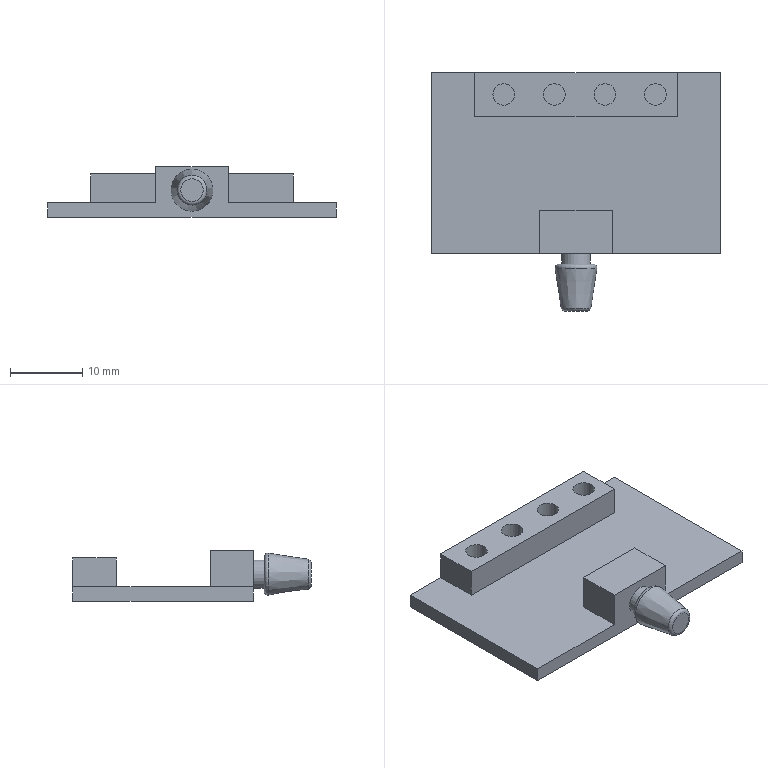Part | NX | features DATUM_CSYS 6, EXTRUDE 5, SKETCH 5, BLEND 2, CHAMFER 1 | 1 solid | 28 faces | box 40 x 33 x 7 mm | volume 3005 mm3 | plane 20 | cylinder 5 | torus 2 | cone 1 | commonest cylinder face diameters 3 x4 4 x1
STEP:
#1=CARTESIAN_POINT('',(-20.,12.5,2.));
#2=VERTEX_POINT('',#1);
#3=CARTESIAN_POINT('',(-20.,-12.5,2.));
#4=VERTEX_POINT('',#3);
#5=CARTESIAN_POINT('',(-20.,12.5,2.));
#6=DIRECTION('',(0.,-1.,0.));
#7=VECTOR('',#6,1000.);
#8=LINE('',#5,#7);
#9=EDGE_CURVE('',#2,#4,#8,.T.);
#10=ORIENTED_EDGE('',*,*,#9,.F.);
#11=CARTESIAN_POINT('',(-20.,12.5,0.));
#12=VERTEX_POINT('',#11);
#13=CARTESIAN_POINT('',(-20.,12.5,0.));
#14=DIRECTION('',(0.,0.,1.));
#15=VECTOR('',#14,1000.);
#16=LINE('',#13,#15);
#17=EDGE_CURVE('',#12,#2,#16,.T.);
#18=ORIENTED_EDGE('',*,*,#17,.F.);
#19=CARTESIAN_POINT('',(-20.,-12.5,0.));
#20=VERTEX_POINT('',#19);
#21=CARTESIAN_POINT('',(-20.,12.5,0.));
#22=DIRECTION('',(0.,-1.,0.));
#23=VECTOR('',#22,1000.);
#24=LINE('',#21,#23);
#25=EDGE_CURVE('',#12,#20,#24,.T.);
#26=ORIENTED_EDGE('',*,*,#25,.T.);
#27=CARTESIAN_POINT('',(-20.,-12.5,0.));
#28=DIRECTION('',(0.,0.,1.));
#29=VECTOR('',#28,1000.);
#30=LINE('',#27,#29);
#31=EDGE_CURVE('',#20,#4,#30,.T.);
#32=ORIENTED_EDGE('',*,*,#31,.T.);
#33=EDGE_LOOP('',(#10,#18,#26,#32));
#34=FACE_BOUND('',#33,.T.);
#35=CARTESIAN_POINT('',(-20.,12.5,0.));
#36=DIRECTION('',(-1.,0.,0.));
#37=DIRECTION('',(0.,-1.,0.));
#38=AXIS2_PLACEMENT_3D('',#35,#36,#37);
#39=PLANE('',#38);
#40=ADVANCED_FACE('',(#34),#39,.T.);
#41=CARTESIAN_POINT('',(-5.,-12.5,2.));
#42=VERTEX_POINT('',#41);
#43=CARTESIAN_POINT('',(-20.,-12.5,2.));
#44=DIRECTION('',(1.,0.,0.));
#45=VECTOR('',#44,1000.);
#46=LINE('',#43,#45);
#47=EDGE_CURVE('',#4,#42,#46,.T.);
#48=ORIENTED_EDGE('',*,*,#47,.F.);
#49=ORIENTED_EDGE('',*,*,#31,.F.);
#50=CARTESIAN_POINT('',(20.,-12.5,0.));
#51=VERTEX_POINT('',#50);
#52=CARTESIAN_POINT('',(-20.,-12.5,0.));
#53=DIRECTION('',(1.,0.,0.));
#54=VECTOR('',#53,1000.);
#55=LINE('',#52,#54);
#56=EDGE_CURVE('',#20,#51,#55,.T.);
#57=ORIENTED_EDGE('',*,*,#56,.T.);
#58=CARTESIAN_POINT('',(20.,-12.5,2.));
#59=VERTEX_POINT('',#58);
#60=CARTESIAN_POINT('',(20.,-12.5,0.));
#61=DIRECTION('',(0.,0.,1.));
#62=VECTOR('',#61,1000.);
#63=LINE('',#60,#62);
#64=EDGE_CURVE('',#51,#59,#63,.T.);
#65=ORIENTED_EDGE('',*,*,#64,.T.);
#66=CARTESIAN_POINT('',(5.,-12.5,2.));
#67=VERTEX_POINT('',#66);
#68=CARTESIAN_POINT('',(-20.,-12.5,2.));
#69=DIRECTION('',(1.,0.,0.));
#70=VECTOR('',#69,1000.);
#71=LINE('',#68,#70);
#72=EDGE_CURVE('',#67,#59,#71,.T.);
#73=ORIENTED_EDGE('',*,*,#72,.F.);
#74=CARTESIAN_POINT('',(5.,-12.5,7.));
#75=VERTEX_POINT('',#74);
#76=CARTESIAN_POINT('',(5.,-12.5,2.));
#77=DIRECTION('',(0.,0.,1.));
#78=VECTOR('',#77,1000.);
#79=LINE('',#76,#78);
#80=EDGE_CURVE('',#67,#75,#79,.T.);
#81=ORIENTED_EDGE('',*,*,#80,.T.);
#82=CARTESIAN_POINT('',(-5.,-12.5,7.));
#83=VERTEX_POINT('',#82);
#84=CARTESIAN_POINT('',(-5.,-12.5,7.));
#85=DIRECTION('',(1.,0.,0.));
#86=VECTOR('',#85,1000.);
#87=LINE('',#84,#86);
#88=EDGE_CURVE('',#83,#75,#87,.T.);
#89=ORIENTED_EDGE('',*,*,#88,.F.);
#90=CARTESIAN_POINT('',(-5.,-12.5,2.));
#91=DIRECTION('',(0.,0.,1.));
#92=VECTOR('',#91,1000.);
#93=LINE('',#90,#92);
#94=EDGE_CURVE('',#42,#83,#93,.T.);
#95=ORIENTED_EDGE('',*,*,#94,.F.);
#96=EDGE_LOOP('',(#48,#49,#57,#65,#73,#81,#89,#95));
#97=FACE_BOUND('',#96,.T.);
#98=CARTESIAN_POINT('',(2.,-12.5,3.755));
#99=VERTEX_POINT('',#98);
#100=CARTESIAN_POINT('',(0.,-12.5,3.755));
#101=DIRECTION('',(0.,-1.,0.));
#102=DIRECTION('',(1.,0.,0.));
#103=AXIS2_PLACEMENT_3D('',#100,#101,#102);
#104=CIRCLE('',#103,2.);
#105=EDGE_CURVE('',#99,#99,#104,.T.);
#106=ORIENTED_EDGE('',*,*,#105,.F.);
#107=EDGE_LOOP('',(#106));
#108=FACE_BOUND('',#107,.T.);
#109=CARTESIAN_POINT('',(-20.,-12.5,0.));
#110=DIRECTION('',(0.,-1.,0.));
#111=DIRECTION('',(0.,0.,-1.));
#112=AXIS2_PLACEMENT_3D('',#109,#110,#111);
#113=PLANE('',#112);
#114=ADVANCED_FACE('',(#97,#108),#113,.T.);
#115=CARTESIAN_POINT('',(20.,12.5,2.));
#116=VERTEX_POINT('',#115);
#117=CARTESIAN_POINT('',(20.,-12.5,2.));
#118=DIRECTION('',(0.,1.,0.));
#119=VECTOR('',#118,1000.);
#120=LINE('',#117,#119);
#121=EDGE_CURVE('',#59,#116,#120,.T.);
#122=ORIENTED_EDGE('',*,*,#121,.F.);
#123=ORIENTED_EDGE('',*,*,#64,.F.);
#124=CARTESIAN_POINT('',(20.,12.5,0.));
#125=VERTEX_POINT('',#124);
#126=CARTESIAN_POINT('',(20.,-12.5,0.));
#127=DIRECTION('',(0.,1.,0.));
#128=VECTOR('',#127,1000.);
#129=LINE('',#126,#128);
#130=EDGE_CURVE('',#51,#125,#129,.T.);
#131=ORIENTED_EDGE('',*,*,#130,.T.);
#132=CARTESIAN_POINT('',(20.,12.5,0.));
#133=DIRECTION('',(0.,0.,1.));
#134=VECTOR('',#133,1000.);
#135=LINE('',#132,#134);
#136=EDGE_CURVE('',#125,#116,#135,.T.);
#137=ORIENTED_EDGE('',*,*,#136,.T.);
#138=EDGE_LOOP('',(#122,#123,#131,#137));
#139=FACE_BOUND('',#138,.T.);
#140=CARTESIAN_POINT('',(20.,-12.5,0.));
#141=DIRECTION('',(1.,0.,0.));
#142=DIRECTION('',(0.,0.,-1.));
#143=AXIS2_PLACEMENT_3D('',#140,#141,#142);
#144=PLANE('',#143);
#145=ADVANCED_FACE('',(#139),#144,.T.);
#146=CARTESIAN_POINT('',(14.,12.5,2.));
#147=VERTEX_POINT('',#146);
#148=CARTESIAN_POINT('',(20.,12.5,2.));
#149=DIRECTION('',(-1.,0.,0.));
#150=VECTOR('',#149,1000.);
#151=LINE('',#148,#150);
#152=EDGE_CURVE('',#116,#147,#151,.T.);
#153=ORIENTED_EDGE('',*,*,#152,.F.);
#154=ORIENTED_EDGE('',*,*,#136,.F.);
#155=CARTESIAN_POINT('',(20.,12.5,0.));
#156=DIRECTION('',(-1.,0.,0.));
#157=VECTOR('',#156,1000.);
#158=LINE('',#155,#157);
#159=EDGE_CURVE('',#125,#12,#158,.T.);
#160=ORIENTED_EDGE('',*,*,#159,.T.);
#161=ORIENTED_EDGE('',*,*,#17,.T.);
#162=CARTESIAN_POINT('',(-14.,12.5,2.));
#163=VERTEX_POINT('',#162);
#164=CARTESIAN_POINT('',(20.,12.5,2.));
#165=DIRECTION('',(-1.,0.,0.));
#166=VECTOR('',#165,1000.);
#167=LINE('',#164,#166);
#168=EDGE_CURVE('',#163,#2,#167,.T.);
#169=ORIENTED_EDGE('',*,*,#168,.F.);
#170=CARTESIAN_POINT('',(-14.,12.5,6.));
#171=VERTEX_POINT('',#170);
#172=CARTESIAN_POINT('',(-14.,12.5,2.));
#173=DIRECTION('',(0.,0.,1.));
#174=VECTOR('',#173,1000.);
#175=LINE('',#172,#174);
#176=EDGE_CURVE('',#163,#171,#175,.T.);
#177=ORIENTED_EDGE('',*,*,#176,.T.);
#178=CARTESIAN_POINT('',(14.,12.5,6.));
#179=VERTEX_POINT('',#178);
#180=CARTESIAN_POINT('',(14.,12.5,6.));
#181=DIRECTION('',(-1.,0.,0.));
#182=VECTOR('',#181,1000.);
#183=LINE('',#180,#182);
#184=EDGE_CURVE('',#179,#171,#183,.T.);
#185=ORIENTED_EDGE('',*,*,#184,.F.);
#186=CARTESIAN_POINT('',(14.,12.5,2.));
#187=DIRECTION('',(0.,0.,1.));
#188=VECTOR('',#187,1000.);
#189=LINE('',#186,#188);
#190=EDGE_CURVE('',#147,#179,#189,.T.);
#191=ORIENTED_EDGE('',*,*,#190,.F.);
#192=EDGE_LOOP('',(#153,#154,#160,#161,#169,#177,#185,#191));
#193=FACE_BOUND('',#192,.T.);
#194=CARTESIAN_POINT('',(20.,12.5,0.));
#195=DIRECTION('',(0.,1.,0.));
#196=DIRECTION('',(-1.,0.,0.));
#197=AXIS2_PLACEMENT_3D('',#194,#195,#196);
#198=PLANE('',#197);
#199=ADVANCED_FACE('',(#193),#198,.T.);
#200=ORIENTED_EDGE('',*,*,#25,.F.);
#201=ORIENTED_EDGE('',*,*,#159,.F.);
#202=ORIENTED_EDGE('',*,*,#130,.F.);
#203=ORIENTED_EDGE('',*,*,#56,.F.);
#204=EDGE_LOOP('',(#200,#201,#202,#203));
#205=FACE_BOUND('',#204,.T.);
#206=CARTESIAN_POINT('',(0.,0.,0.));
#207=DIRECTION('',(0.,0.,1.));
#208=DIRECTION('',(1.,0.,0.));
#209=AXIS2_PLACEMENT_3D('',#206,#207,#208);
#210=PLANE('',#209);
#211=ADVANCED_FACE('',(#205),#210,.F.);
#212=CARTESIAN_POINT('',(-5.,-6.5,2.));
#213=VERTEX_POINT('',#212);
#214=CARTESIAN_POINT('',(-5.,-6.5,2.));
#215=DIRECTION('',(0.,-1.,0.));
#216=VECTOR('',#215,1000.);
#217=LINE('',#214,#216);
#218=EDGE_CURVE('',#213,#42,#217,.T.);
#219=ORIENTED_EDGE('',*,*,#218,.F.);
#220=CARTESIAN_POINT('',(5.,-6.5,2.));
#221=VERTEX_POINT('',#220);
#222=CARTESIAN_POINT('',(5.,-6.5,2.));
#223=DIRECTION('',(-1.,0.,0.));
#224=VECTOR('',#223,1000.);
#225=LINE('',#222,#224);
#226=EDGE_CURVE('',#221,#213,#225,.T.);
#227=ORIENTED_EDGE('',*,*,#226,.F.);
#228=CARTESIAN_POINT('',(5.,-12.5,2.));
#229=DIRECTION('',(0.,1.,0.));
#230=VECTOR('',#229,1000.);
#231=LINE('',#228,#230);
#232=EDGE_CURVE('',#67,#221,#231,.T.);
#233=ORIENTED_EDGE('',*,*,#232,.F.);
#234=ORIENTED_EDGE('',*,*,#72,.T.);
#235=ORIENTED_EDGE('',*,*,#121,.T.);
#236=ORIENTED_EDGE('',*,*,#152,.T.);
#237=CARTESIAN_POINT('',(14.,6.5,2.));
#238=VERTEX_POINT('',#237);
#239=CARTESIAN_POINT('',(14.,6.5,2.));
#240=DIRECTION('',(0.,1.,0.));
#241=VECTOR('',#240,1000.);
#242=LINE('',#239,#241);
#243=EDGE_CURVE('',#238,#147,#242,.T.);
#244=ORIENTED_EDGE('',*,*,#243,.F.);
#245=CARTESIAN_POINT('',(-14.,6.5,2.));
#246=VERTEX_POINT('',#245);
#247=CARTESIAN_POINT('',(-14.,6.5,2.));
#248=DIRECTION('',(1.,0.,0.));
#249=VECTOR('',#248,1000.);
#250=LINE('',#247,#249);
#251=EDGE_CURVE('',#246,#238,#250,.T.);
#252=ORIENTED_EDGE('',*,*,#251,.F.);
#253=CARTESIAN_POINT('',(-14.,12.5,2.));
#254=DIRECTION('',(0.,-1.,0.));
#255=VECTOR('',#254,1000.);
#256=LINE('',#253,#255);
#257=EDGE_CURVE('',#163,#246,#256,.T.);
#258=ORIENTED_EDGE('',*,*,#257,.F.);
#259=ORIENTED_EDGE('',*,*,#168,.T.);
#260=ORIENTED_EDGE('',*,*,#9,.T.);
#261=ORIENTED_EDGE('',*,*,#47,.T.);
#262=EDGE_LOOP('',(#219,#227,#233,#234,#235,#236,#244,#252,#258,#259,#260,#261));
#263=FACE_BOUND('',#262,.T.);
#264=CARTESIAN_POINT('',(0.,0.,2.));
#265=DIRECTION('',(0.,0.,1.));
#266=DIRECTION('',(1.,0.,0.));
#267=AXIS2_PLACEMENT_3D('',#264,#265,#266);
#268=PLANE('',#267);
#269=ADVANCED_FACE('',(#263),#268,.T.);
#270=CARTESIAN_POINT('',(-14.,6.5,6.));
#271=VERTEX_POINT('',#270);
#272=CARTESIAN_POINT('',(-14.,12.5,6.));
#273=DIRECTION('',(0.,-1.,0.));
#274=VECTOR('',#273,1000.);
#275=LINE('',#272,#274);
#276=EDGE_CURVE('',#171,#271,#275,.T.);
#277=ORIENTED_EDGE('',*,*,#276,.F.);
#278=ORIENTED_EDGE('',*,*,#176,.F.);
#279=ORIENTED_EDGE('',*,*,#257,.T.);
#280=CARTESIAN_POINT('',(-14.,6.5,2.));
#281=DIRECTION('',(0.,0.,1.));
#282=VECTOR('',#281,1000.);
#283=LINE('',#280,#282);
#284=EDGE_CURVE('',#246,#271,#283,.T.);
#285=ORIENTED_EDGE('',*,*,#284,.T.);
#286=EDGE_LOOP('',(#277,#278,#279,#285));
#287=FACE_BOUND('',#286,.T.);
#288=CARTESIAN_POINT('',(-14.,12.5,2.));
#289=DIRECTION('',(-1.,0.,0.));
#290=DIRECTION('',(0.,0.,1.));
#291=AXIS2_PLACEMENT_3D('',#288,#289,#290);
#292=PLANE('',#291);
#293=ADVANCED_FACE('',(#287),#292,.T.);
#294=CARTESIAN_POINT('',(14.,6.5,6.));
#295=VERTEX_POINT('',#294);
#296=CARTESIAN_POINT('',(-14.,6.5,6.));
#297=DIRECTION('',(1.,0.,0.));
#298=VECTOR('',#297,1000.);
#299=LINE('',#296,#298);
#300=EDGE_CURVE('',#271,#295,#299,.T.);
#301=ORIENTED_EDGE('',*,*,#300,.F.);
#302=ORIENTED_EDGE('',*,*,#284,.F.);
#303=ORIENTED_EDGE('',*,*,#251,.T.);
#304=CARTESIAN_POINT('',(14.,6.5,2.));
#305=DIRECTION('',(0.,0.,1.));
#306=VECTOR('',#305,1000.);
#307=LINE('',#304,#306);
#308=EDGE_CURVE('',#238,#295,#307,.T.);
#309=ORIENTED_EDGE('',*,*,#308,.T.);
#310=EDGE_LOOP('',(#301,#302,#303,#309));
#311=FACE_BOUND('',#310,.T.);
#312=CARTESIAN_POINT('',(-14.,6.5,2.));
#313=DIRECTION('',(0.,-1.,0.));
#314=DIRECTION('',(0.,0.,-1.));
#315=AXIS2_PLACEMENT_3D('',#312,#313,#314);
#316=PLANE('',#315);
#317=ADVANCED_FACE('',(#311),#316,.T.);
#318=CARTESIAN_POINT('',(14.,6.5,6.));
#319=DIRECTION('',(0.,1.,0.));
#320=VECTOR('',#319,1000.);
#321=LINE('',#318,#320);
#322=EDGE_CURVE('',#295,#179,#321,.T.);
#323=ORIENTED_EDGE('',*,*,#322,.F.);
#324=ORIENTED_EDGE('',*,*,#308,.F.);
#325=ORIENTED_EDGE('',*,*,#243,.T.);
#326=ORIENTED_EDGE('',*,*,#190,.T.);
#327=EDGE_LOOP('',(#323,#324,#325,#326));
#328=FACE_BOUND('',#327,.T.);
#329=CARTESIAN_POINT('',(14.,6.5,2.));
#330=DIRECTION('',(1.,0.,0.));
#331=DIRECTION('',(0.,0.,-1.));
#332=AXIS2_PLACEMENT_3D('',#329,#330,#331);
#333=PLANE('',#332);
#334=ADVANCED_FACE('',(#328),#333,.T.);
#335=CARTESIAN_POINT('',(5.5,9.5,2.));
#336=VERTEX_POINT('',#335);
#337=CARTESIAN_POINT('',(4.,9.5,2.));
#338=DIRECTION('',(0.,0.,1.));
#339=DIRECTION('',(1.,0.,0.));
#340=AXIS2_PLACEMENT_3D('',#337,#338,#339);
#341=CIRCLE('',#340,1.5);
#342=EDGE_CURVE('',#336,#336,#341,.T.);
#343=ORIENTED_EDGE('',*,*,#342,.F.);
#344=EDGE_LOOP('',(#343));
#345=FACE_BOUND('',#344,.T.);
#346=CARTESIAN_POINT('',(5.5,9.5,6.));
#347=VERTEX_POINT('',#346);
#348=CARTESIAN_POINT('',(4.,9.5,6.));
#349=DIRECTION('',(0.,0.,1.));
#350=DIRECTION('',(1.,0.,0.));
#351=AXIS2_PLACEMENT_3D('',#348,#349,#350);
#352=CIRCLE('',#351,1.5);
#353=EDGE_CURVE('',#347,#347,#352,.T.);
#354=ORIENTED_EDGE('',*,*,#353,.T.);
#355=EDGE_LOOP('',(#354));
#356=FACE_BOUND('',#355,.T.);
#357=CARTESIAN_POINT('',(4.,9.5,2.));
#358=DIRECTION('',(0.,0.,1.));
#359=DIRECTION('',(1.,0.,0.));
#360=AXIS2_PLACEMENT_3D('',#357,#358,#359);
#361=CYLINDRICAL_SURFACE('',#360,1.5);
#362=ADVANCED_FACE('',(#345,#356),#361,.F.);
#363=CARTESIAN_POINT('',(-1.5,9.5,2.));
#364=VERTEX_POINT('',#363);
#365=CARTESIAN_POINT('',(-3.,9.5,2.));
#366=DIRECTION('',(0.,0.,1.));
#367=DIRECTION('',(1.,0.,0.));
#368=AXIS2_PLACEMENT_3D('',#365,#366,#367);
#369=CIRCLE('',#368,1.5);
#370=EDGE_CURVE('',#364,#364,#369,.T.);
#371=ORIENTED_EDGE('',*,*,#370,.F.);
#372=EDGE_LOOP('',(#371));
#373=FACE_BOUND('',#372,.T.);
#374=CARTESIAN_POINT('',(-1.5,9.5,6.));
#375=VERTEX_POINT('',#374);
#376=CARTESIAN_POINT('',(-3.,9.5,6.));
#377=DIRECTION('',(0.,0.,1.));
#378=DIRECTION('',(1.,0.,0.));
#379=AXIS2_PLACEMENT_3D('',#376,#377,#378);
#380=CIRCLE('',#379,1.5);
#381=EDGE_CURVE('',#375,#375,#380,.T.);
#382=ORIENTED_EDGE('',*,*,#381,.T.);
#383=EDGE_LOOP('',(#382));
#384=FACE_BOUND('',#383,.T.);
#385=CARTESIAN_POINT('',(-3.,9.5,2.));
#386=DIRECTION('',(0.,0.,1.));
#387=DIRECTION('',(1.,0.,0.));
#388=AXIS2_PLACEMENT_3D('',#385,#386,#387);
#389=CYLINDRICAL_SURFACE('',#388,1.5);
#390=ADVANCED_FACE('',(#373,#384),#389,.F.);
#391=CARTESIAN_POINT('',(-8.5,9.5,2.));
#392=VERTEX_POINT('',#391);
#393=CARTESIAN_POINT('',(-10.,9.5,2.));
#394=DIRECTION('',(0.,0.,1.));
#395=DIRECTION('',(1.,0.,0.));
#396=AXIS2_PLACEMENT_3D('',#393,#394,#395);
#397=CIRCLE('',#396,1.5);
#398=EDGE_CURVE('',#392,#392,#397,.T.);
#399=ORIENTED_EDGE('',*,*,#398,.F.);
#400=EDGE_LOOP('',(#399));
#401=FACE_BOUND('',#400,.T.);
#402=CARTESIAN_POINT('',(-8.5,9.5,6.));
#403=VERTEX_POINT('',#402);
#404=CARTESIAN_POINT('',(-10.,9.5,6.));
#405=DIRECTION('',(0.,0.,1.));
#406=DIRECTION('',(1.,0.,0.));
#407=AXIS2_PLACEMENT_3D('',#404,#405,#406);
#408=CIRCLE('',#407,1.5);
#409=EDGE_CURVE('',#403,#403,#408,.T.);
#410=ORIENTED_EDGE('',*,*,#409,.T.);
#411=EDGE_LOOP('',(#410));
#412=FACE_BOUND('',#411,.T.);
#413=CARTESIAN_POINT('',(-10.,9.5,2.));
#414=DIRECTION('',(0.,0.,1.));
#415=DIRECTION('',(1.,0.,0.));
#416=AXIS2_PLACEMENT_3D('',#413,#414,#415);
#417=CYLINDRICAL_SURFACE('',#416,1.5);
#418=ADVANCED_FACE('',(#401,#412),#417,.F.);
#419=CARTESIAN_POINT('',(12.5,9.5,2.));
#420=VERTEX_POINT('',#419);
#421=CARTESIAN_POINT('',(11.,9.5,2.));
#422=DIRECTION('',(0.,0.,1.));
#423=DIRECTION('',(1.,0.,0.));
#424=AXIS2_PLACEMENT_3D('',#421,#422,#423);
#425=CIRCLE('',#424,1.5);
#426=EDGE_CURVE('',#420,#420,#425,.T.);
#427=ORIENTED_EDGE('',*,*,#426,.F.);
#428=EDGE_LOOP('',(#427));
#429=FACE_BOUND('',#428,.T.);
#430=CARTESIAN_POINT('',(12.5,9.5,6.));
#431=VERTEX_POINT('',#430);
#432=CARTESIAN_POINT('',(11.,9.5,6.));
#433=DIRECTION('',(0.,0.,1.));
#434=DIRECTION('',(1.,0.,0.));
#435=AXIS2_PLACEMENT_3D('',#432,#433,#434);
#436=CIRCLE('',#435,1.5);
#437=EDGE_CURVE('',#431,#431,#436,.T.);
#438=ORIENTED_EDGE('',*,*,#437,.T.);
#439=EDGE_LOOP('',(#438));
#440=FACE_BOUND('',#439,.T.);
#441=CARTESIAN_POINT('',(11.,9.5,2.));
#442=DIRECTION('',(0.,0.,1.));
#443=DIRECTION('',(1.,0.,0.));
#444=AXIS2_PLACEMENT_3D('',#441,#442,#443);
#445=CYLINDRICAL_SURFACE('',#444,1.5);
#446=ADVANCED_FACE('',(#429,#440),#445,.F.);
#447=ORIENTED_EDGE('',*,*,#276,.T.);
#448=ORIENTED_EDGE('',*,*,#300,.T.);
#449=ORIENTED_EDGE('',*,*,#322,.T.);
#450=ORIENTED_EDGE('',*,*,#184,.T.);
#451=EDGE_LOOP('',(#447,#448,#449,#450));
#452=FACE_BOUND('',#451,.T.);
#453=ORIENTED_EDGE('',*,*,#409,.F.);
#454=EDGE_LOOP('',(#453));
#455=FACE_BOUND('',#454,.T.);
#456=ORIENTED_EDGE('',*,*,#381,.F.);
#457=EDGE_LOOP('',(#456));
#458=FACE_BOUND('',#457,.T.);
#459=ORIENTED_EDGE('',*,*,#353,.F.);
#460=EDGE_LOOP('',(#459));
#461=FACE_BOUND('',#460,.T.);
#462=ORIENTED_EDGE('',*,*,#437,.F.);
#463=EDGE_LOOP('',(#462));
#464=FACE_BOUND('',#463,.T.);
#465=CARTESIAN_POINT('',(-10.,9.5,6.));
#466=DIRECTION('',(0.,0.,1.));
#467=DIRECTION('',(1.,0.,0.));
#468=AXIS2_PLACEMENT_3D('',#465,#466,#467);
#469=PLANE('',#468);
#470=ADVANCED_FACE('',(#452,#455,#458,#461,#464),#469,.T.);
#471=ORIENTED_EDGE('',*,*,#342,.T.);
#472=EDGE_LOOP('',(#471));
#473=FACE_BOUND('',#472,.T.);
#474=CARTESIAN_POINT('',(0.,0.,2.));
#475=DIRECTION('',(0.,0.,1.));
#476=DIRECTION('',(1.,0.,0.));
#477=AXIS2_PLACEMENT_3D('',#474,#475,#476);
#478=PLANE('',#477);
#479=ADVANCED_FACE('',(#473),#478,.T.);
#480=ORIENTED_EDGE('',*,*,#370,.T.);
#481=EDGE_LOOP('',(#480));
#482=FACE_BOUND('',#481,.T.);
#483=CARTESIAN_POINT('',(0.,0.,2.));
#484=DIRECTION('',(0.,0.,1.));
#485=DIRECTION('',(1.,0.,0.));
#486=AXIS2_PLACEMENT_3D('',#483,#484,#485);
#487=PLANE('',#486);
#488=ADVANCED_FACE('',(#482),#487,.T.);
#489=ORIENTED_EDGE('',*,*,#398,.T.);
#490=EDGE_LOOP('',(#489));
#491=FACE_BOUND('',#490,.T.);
#492=CARTESIAN_POINT('',(0.,0.,2.));
#493=DIRECTION('',(0.,0.,1.));
#494=DIRECTION('',(1.,0.,0.));
#495=AXIS2_PLACEMENT_3D('',#492,#493,#494);
#496=PLANE('',#495);
#497=ADVANCED_FACE('',(#491),#496,.T.);
#498=ORIENTED_EDGE('',*,*,#426,.T.);
#499=EDGE_LOOP('',(#498));
#500=FACE_BOUND('',#499,.T.);
#501=CARTESIAN_POINT('',(0.,0.,2.));
#502=DIRECTION('',(0.,0.,1.));
#503=DIRECTION('',(1.,0.,0.));
#504=AXIS2_PLACEMENT_3D('',#501,#502,#503);
#505=PLANE('',#504);
#506=ADVANCED_FACE('',(#500),#505,.T.);
#507=CARTESIAN_POINT('',(-5.,-6.5,7.));
#508=VERTEX_POINT('',#507);
#509=CARTESIAN_POINT('',(-5.,-6.5,7.));
#510=DIRECTION('',(0.,-1.,0.));
#511=VECTOR('',#510,1000.);
#512=LINE('',#509,#511);
#513=EDGE_CURVE('',#508,#83,#512,.T.);
#514=ORIENTED_EDGE('',*,*,#513,.F.);
#515=CARTESIAN_POINT('',(-5.,-6.5,2.));
#516=DIRECTION('',(0.,0.,1.));
#517=VECTOR('',#516,1000.);
#518=LINE('',#515,#517);
#519=EDGE_CURVE('',#213,#508,#518,.T.);
#520=ORIENTED_EDGE('',*,*,#519,.F.);
#521=ORIENTED_EDGE('',*,*,#218,.T.);
#522=ORIENTED_EDGE('',*,*,#94,.T.);
#523=EDGE_LOOP('',(#514,#520,#521,#522));
#524=FACE_BOUND('',#523,.T.);
#525=CARTESIAN_POINT('',(-5.,-6.5,2.));
#526=DIRECTION('',(-1.,0.,0.));
#527=DIRECTION('',(0.,-1.,0.));
#528=AXIS2_PLACEMENT_3D('',#525,#526,#527);
#529=PLANE('',#528);
#530=ADVANCED_FACE('',(#524),#529,.T.);
#531=CARTESIAN_POINT('',(5.,-6.5,7.));
#532=VERTEX_POINT('',#531);
#533=CARTESIAN_POINT('',(5.,-12.5,7.));
#534=DIRECTION('',(0.,1.,0.));
#535=VECTOR('',#534,1000.);
#536=LINE('',#533,#535);
#537=EDGE_CURVE('',#75,#532,#536,.T.);
#538=ORIENTED_EDGE('',*,*,#537,.F.);
#539=ORIENTED_EDGE('',*,*,#80,.F.);
#540=ORIENTED_EDGE('',*,*,#232,.T.);
#541=CARTESIAN_POINT('',(5.,-6.5,2.));
#542=DIRECTION('',(0.,0.,1.));
#543=VECTOR('',#542,1000.);
#544=LINE('',#541,#543);
#545=EDGE_CURVE('',#221,#532,#544,.T.);
#546=ORIENTED_EDGE('',*,*,#545,.T.);
#547=EDGE_LOOP('',(#538,#539,#540,#546));
#548=FACE_BOUND('',#547,.T.);
#549=CARTESIAN_POINT('',(5.,-12.5,2.));
#550=DIRECTION('',(1.,0.,0.));
#551=DIRECTION('',(0.,0.,-1.));
#552=AXIS2_PLACEMENT_3D('',#549,#550,#551);
#553=PLANE('',#552);
#554=ADVANCED_FACE('',(#548),#553,.T.);
#555=CARTESIAN_POINT('',(5.,-6.5,7.));
#556=DIRECTION('',(-1.,0.,0.));
#557=VECTOR('',#556,1000.);
#558=LINE('',#555,#557);
#559=EDGE_CURVE('',#532,#508,#558,.T.);
#560=ORIENTED_EDGE('',*,*,#559,.F.);
#561=ORIENTED_EDGE('',*,*,#545,.F.);
#562=ORIENTED_EDGE('',*,*,#226,.T.);
#563=ORIENTED_EDGE('',*,*,#519,.T.);
#564=EDGE_LOOP('',(#560,#561,#562,#563));
#565=FACE_BOUND('',#564,.T.);
#566=CARTESIAN_POINT('',(5.,-6.5,2.));
#567=DIRECTION('',(0.,1.,0.));
#568=DIRECTION('',(-1.,0.,0.));
#569=AXIS2_PLACEMENT_3D('',#566,#567,#568);
#570=PLANE('',#569);
#571=ADVANCED_FACE('',(#565),#570,.T.);
#572=ORIENTED_EDGE('',*,*,#513,.T.);
#573=ORIENTED_EDGE('',*,*,#88,.T.);
#574=ORIENTED_EDGE('',*,*,#537,.T.);
#575=ORIENTED_EDGE('',*,*,#559,.T.);
#576=EDGE_LOOP('',(#572,#573,#574,#575));
#577=FACE_BOUND('',#576,.T.);
#578=CARTESIAN_POINT('',(0.,0.,7.));
#579=DIRECTION('',(0.,0.,1.));
#580=DIRECTION('',(1.,0.,0.));
#581=AXIS2_PLACEMENT_3D('',#578,#579,#580);
#582=PLANE('',#581);
#583=ADVANCED_FACE('',(#577),#582,.T.);
#584=ORIENTED_EDGE('',*,*,#105,.T.);
#585=EDGE_LOOP('',(#584));
#586=FACE_BOUND('',#585,.T.);
#587=CARTESIAN_POINT('',(2.,-14.,3.755));
#588=VERTEX_POINT('',#587);
#589=CARTESIAN_POINT('',(0.,-14.,3.755));
#590=DIRECTION('',(0.,-1.,0.));
#591=DIRECTION('',(1.,0.,0.));
#592=AXIS2_PLACEMENT_3D('',#589,#590,#591);
#593=CIRCLE('',#592,2.);
#594=EDGE_CURVE('',#588,#588,#593,.F.);
#595=ORIENTED_EDGE('',*,*,#594,.T.);
#596=EDGE_LOOP('',(#595));
#597=FACE_BOUND('',#596,.T.);
#598=CARTESIAN_POINT('',(0.,-12.5,3.755));
#599=DIRECTION('',(0.,-1.,0.));
#600=DIRECTION('',(0.,0.,-1.));
#601=AXIS2_PLACEMENT_3D('',#598,#599,#600);
#602=CYLINDRICAL_SURFACE('',#601,2.);
#603=ADVANCED_FACE('',(#586,#597),#602,.T.);
#604=CARTESIAN_POINT('',(0.,-14.,1.338));
#605=VERTEX_POINT('',#604);
#606=CARTESIAN_POINT('',(0.,-14.,3.755));
#607=DIRECTION('',(0.,-1.,0.));
#608=DIRECTION('',(0.,0.,-1.));
#609=AXIS2_PLACEMENT_3D('',#606,#607,#608);
#610=CIRCLE('',#609,2.417);
#611=EDGE_CURVE('',#605,#605,#610,.F.);
#612=ORIENTED_EDGE('',*,*,#611,.T.);
#613=EDGE_LOOP('',(#612));
#614=FACE_BOUND('',#613,.T.);
#615=ORIENTED_EDGE('',*,*,#594,.F.);
#616=EDGE_LOOP('',(#615));
#617=FACE_BOUND('',#616,.T.);
#618=CARTESIAN_POINT('',(0.,-14.,3.755));
#619=DIRECTION('',(0.,-1.,0.));
#620=DIRECTION('',(0.,0.,-1.));
#621=AXIS2_PLACEMENT_3D('',#618,#619,#620);
#622=PLANE('',#621);
#623=ADVANCED_FACE('',(#614,#617),#622,.F.);
#624=CARTESIAN_POINT('',(0.,-20.5,2.184));
#625=VERTEX_POINT('',#624);
#626=CARTESIAN_POINT('',(0.,-20.5,3.755));
#627=DIRECTION('',(0.,-1.,0.));
#628=DIRECTION('',(0.,0.,-1.));
#629=AXIS2_PLACEMENT_3D('',#626,#627,#628);
#630=CIRCLE('',#629,1.571);
#631=EDGE_CURVE('',#625,#625,#630,.T.);
#632=ORIENTED_EDGE('',*,*,#631,.T.);
#633=EDGE_LOOP('',(#632));
#634=FACE_BOUND('',#633,.T.);
#635=CARTESIAN_POINT('',(0.,-20.5,3.755));
#636=DIRECTION('',(0.,-1.,0.));
#637=DIRECTION('',(0.,0.,-1.));
#638=AXIS2_PLACEMENT_3D('',#635,#636,#637);
#639=PLANE('',#638);
#640=ADVANCED_FACE('',(#634),#639,.T.);
#641=CARTESIAN_POINT('',(0.,-20.076,1.69));
#642=VERTEX_POINT('',#641);
#643=CARTESIAN_POINT('',(0.,-20.076,3.755));
#644=DIRECTION('',(0.,-1.,0.));
#645=DIRECTION('',(0.,0.,-1.));
#646=AXIS2_PLACEMENT_3D('',#643,#644,#645);
#647=CIRCLE('',#646,2.065);
#648=EDGE_CURVE('',#642,#642,#647,.F.);
#649=ORIENTED_EDGE('',*,*,#648,.F.);
#650=EDGE_LOOP('',(#649));
#651=FACE_BOUND('',#650,.T.);
#652=ORIENTED_EDGE('',*,*,#631,.F.);
#653=EDGE_LOOP('',(#652));
#654=FACE_BOUND('',#653,.T.);
#655=CARTESIAN_POINT('',(0.,-20.,3.755));
#656=DIRECTION('',(0.,-1.,0.));
#657=DIRECTION('',(0.,0.,-1.));
#658=AXIS2_PLACEMENT_3D('',#655,#656,#657);
#659=TOROIDAL_SURFACE('',#658,1.571,0.5);
#660=ADVANCED_FACE('',(#651,#654),#659,.T.);
#661=CARTESIAN_POINT('',(0.,-14.576,6.667));
#662=VERTEX_POINT('',#661);
#663=CARTESIAN_POINT('',(0.,-14.576,3.755));
#664=DIRECTION('',(0.,1.,0.));
#665=DIRECTION('',(0.,0.,1.));
#666=AXIS2_PLACEMENT_3D('',#663,#664,#665);
#667=CIRCLE('',#666,2.911);
#668=EDGE_CURVE('',#662,#662,#667,.F.);
#669=ORIENTED_EDGE('',*,*,#668,.T.);
#670=EDGE_LOOP('',(#669));
#671=FACE_BOUND('',#670,.T.);
#672=ORIENTED_EDGE('',*,*,#648,.T.);
#673=EDGE_LOOP('',(#672));
#674=FACE_BOUND('',#673,.T.);
#675=CARTESIAN_POINT('',(0.,-20.5,3.755));
#676=DIRECTION('',(0.,1.,0.));
#677=DIRECTION('',(0.,0.,1.));
#678=AXIS2_PLACEMENT_3D('',#675,#676,#677);
#679=CONICAL_SURFACE('',#678,2.,0.1526);
#680=ADVANCED_FACE('',(#671,#674),#679,.T.);
#681=ORIENTED_EDGE('',*,*,#611,.F.);
#682=EDGE_LOOP('',(#681));
#683=FACE_BOUND('',#682,.T.);
#684=ORIENTED_EDGE('',*,*,#668,.F.);
#685=EDGE_LOOP('',(#684));
#686=FACE_BOUND('',#685,.T.);
#687=CARTESIAN_POINT('',(0.,-14.5,3.755));
#688=DIRECTION('',(0.,-1.,0.));
#689=DIRECTION('',(0.,0.,-1.));
#690=AXIS2_PLACEMENT_3D('',#687,#688,#689);
#691=TOROIDAL_SURFACE('',#690,2.417,0.5);
#692=ADVANCED_FACE('',(#683,#686),#691,.T.);
#693=CLOSED_SHELL('',(#40,#114,#145,#199,#211,#269,#293,#317,#334,#362,#390,#418,#446,#470,#479,#488,#497,#506,#530,#554,#571,#583,#603,#623,#640,#660,#680,#692));
#694=MANIFOLD_SOLID_BREP('',#693);
#695=(LENGTH_UNIT()NAMED_UNIT(*)SI_UNIT(.MILLI.,.METRE.));
#696=UNCERTAINTY_MEASURE_WITH_UNIT(LENGTH_MEASURE(0.00001),#695,'','');
#697=(NAMED_UNIT(*)PLANE_ANGLE_UNIT()SI_UNIT($,.RADIAN.));
#698=(NAMED_UNIT(*)SI_UNIT($,.STERADIAN.)SOLID_ANGLE_UNIT());
#699=(GEOMETRIC_REPRESENTATION_CONTEXT(3)GLOBAL_UNCERTAINTY_ASSIGNED_CONTEXT((#696))GLOBAL_UNIT_ASSIGNED_CONTEXT((#695,#697,#698))REPRESENTATION_CONTEXT('',''));
#700=ADVANCED_BREP_SHAPE_REPRESENTATION('',(#694),#699);